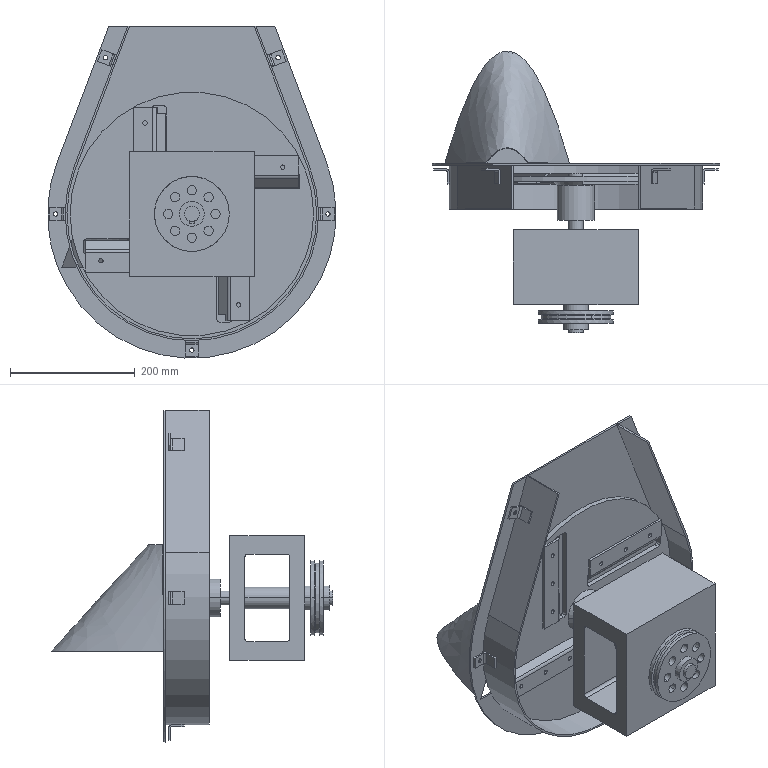Part | SolidWorks | features AEMSimFeature 1 | 50 solids | 616 faces | box 462 x 451 x 532.065 mm | volume 5080659 mm3 | cylinder 214 | plane 210 | sphere 112 | cone 54 | torus 24 | spline 2 | commonest cylinder face diameters 7 x68 10 x36 15 x16 24 x10 40 x10 4 x8